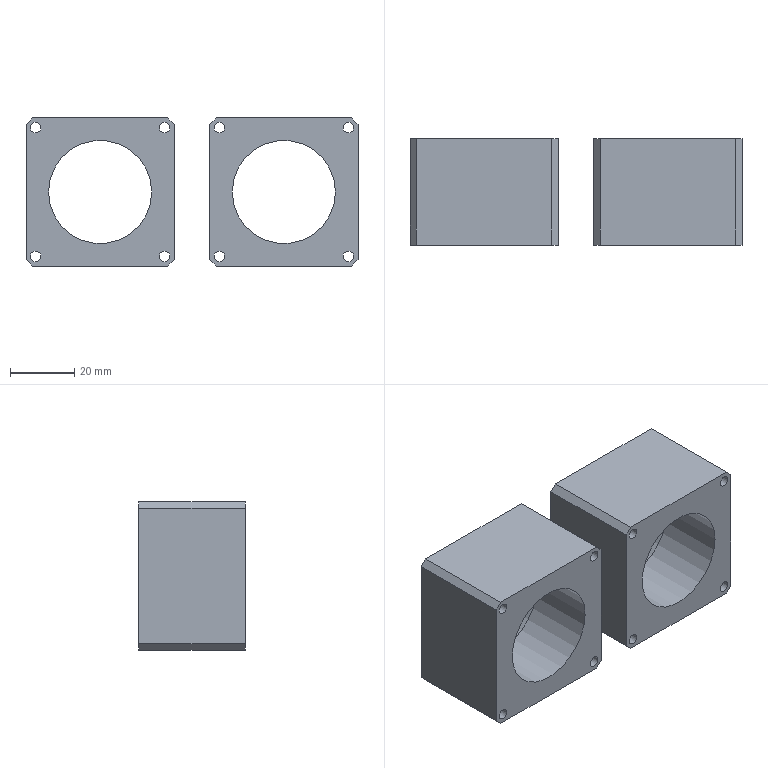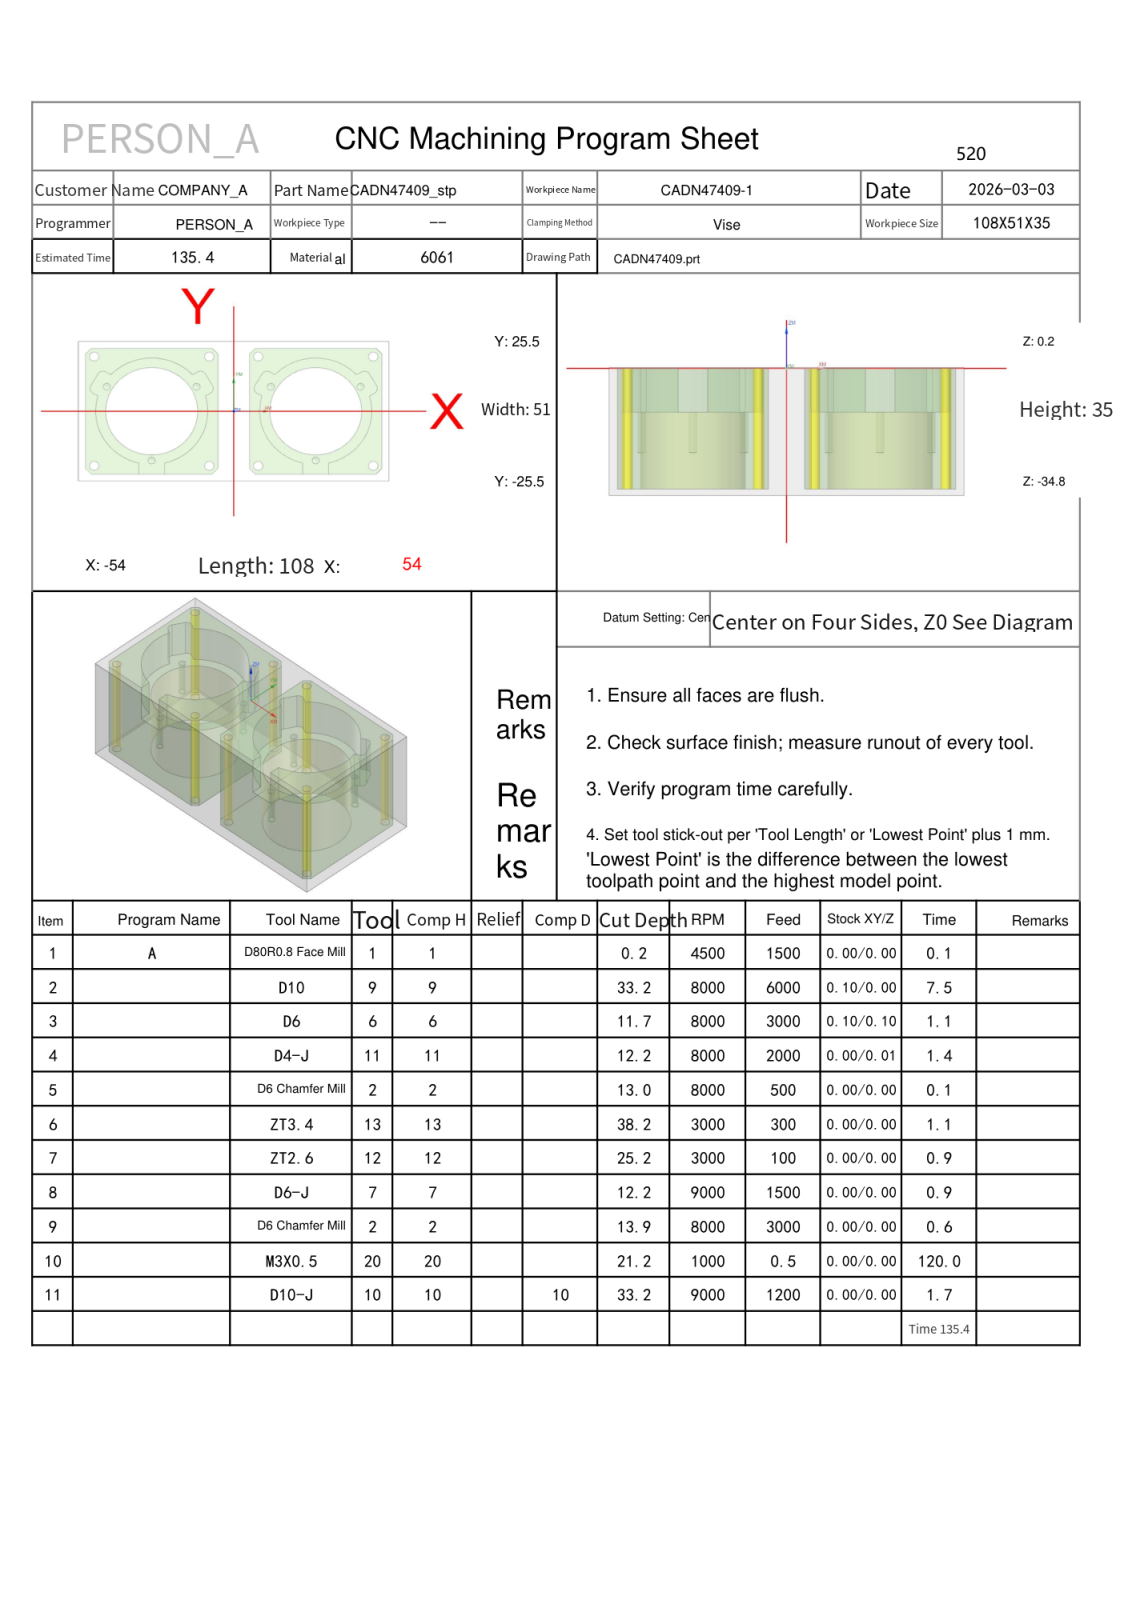NC program | NX | posted by the shop | part box 103 x 33 x 46 mm
Lines 4873 to 5345 of 11287:
N3 T06 M06
(D6  D=6. R=0. H=06 ce=0.10 di=0.10)
G00 G90 G54 X29.9 Y-28.254 M03 S8000
G43 H06 Z50.
M08
Z-.5
G01 Y-23. F3000.
Y-18.974
Y-13.72
G00 Z50.
X27.1
Z-.5
G01 Y-18.974
Y-23.
Y-28.254
G00 Z-1.
G01 Y-23.
Y-18.974
Y-13.72
G00 Z50.
X29.9 Y-28.254
Z-1.
G01 Y-23.
Y-18.974
Y-13.72
G00 Z-1.5
G01 Y-18.974
Y-23.
Y-28.254
G00 Z50.
X27.1 Y-13.72
Z-1.5
G01 Y-18.974
Y-23.
Y-28.254
G00 Z-2.
G01 Y-23.
Y-18.974
Y-13.72
G00 Z50.
X29.9 Y-28.254
Z-2.
G01 Y-23.
Y-18.974
Y-13.72
G00 Z-2.5
G01 Y-18.974
Y-23.
Y-28.254
G00 Z50.
X27.1 Y-13.72
Z-2.5
G01 Y-18.974
Y-23.
Y-28.254
G00 Z-3.
G01 Y-23.
Y-18.974
Y-13.72
G00 Z50.
X29.9 Y-28.254
Z-3.
G01 Y-23.
Y-18.974
Y-13.72
G00 Z-3.5
G01 Y-18.974
Y-23.
Y-28.254
G00 Z50.
X27.1 Y-13.72
Z-3.5
G01 Y-18.974
Y-23.
Y-28.254
G00 Z-4.
G01 Y-23.
Y-18.974
Y-13.72
G00 Z50.
X29.9 Y-28.254
Z-4.
G01 Y-23.
Y-18.974
Y-13.72
G00 Z-4.5
G01 Y-18.974
Y-23.
Y-28.254
G00 Z50.
X27.1 Y-13.72
Z-4.5
G01 Y-18.974
Y-23.
Y-28.254
G00 Z-5.
G01 Y-23.
Y-18.974
Y-13.72
G00 Z50.
X29.9 Y-28.254
Z-5.
G01 Y-23.
Y-18.974
Y-13.72
G00 Z-5.5
G01 Y-18.974
Y-23.
Y-28.254
G00 Z50.
X27.1 Y-13.72
Z-5.5
G01 Y-18.974
Y-23.
Y-28.254
G00 Z-6.
G01 Y-23.
Y-18.974
Y-13.72
G00 Z50.
X29.9 Y-28.254
Z-6.
G01 Y-23.
Y-18.974
Y-13.72
G00 Z-6.5
G01 Y-18.974
Y-23.
Y-28.254
G00 Z50.
X27.1 Y-13.72
Z-6.5
G01 Y-18.974
Y-23.
Y-28.254
G00 Z-7.
G01 Y-23.
Y-18.974
Y-13.72
G00 Z50.
X29.9 Y-28.254
Z-7.
G01 Y-23.
Y-18.974
Y-13.72
G00 Z-7.5
G01 Y-18.974
Y-23.
Y-28.254
G00 Z50.
X27.1 Y-13.72
Z-7.5
G01 Y-18.974
Y-23.
Y-28.254
G00 Z-8.
G01 Y-23.
Y-18.974
Y-13.72
G00 Z50.
X29.9 Y-28.254
Z-8.
G01 Y-23.
Y-18.974
Y-13.72
G00 Z-8.5
G01 Y-18.974
Y-23.
Y-28.254
G00 Z50.
X27.1 Y-13.72
Z-8.5
G01 Y-18.974
Y-23.
Y-28.254
G00 Z-9.
G01 Y-23.
Y-18.974
Y-13.72
G00 Z50.
X29.9 Y-28.254
Z-9.
G01 Y-23.
Y-18.974
Y-13.72
G00 Z-9.5
G01 Y-18.974
Y-23.
Y-28.254
G00 Z50.
X27.1 Y-13.72
Z-9.5
G01 Y-18.974
Y-23.
Y-28.254
G00 Z-10.
G01 Y-23.
Y-18.974
Y-13.72
G00 Z50.
X29.9 Y-28.254
Z-10.
G01 Y-23.
Y-18.974
Y-13.72
G00 Z-10.5
G01 Y-18.974
Y-23.
Y-28.254
G00 Z50.
X27.1 Y-13.72
Z-10.5
G01 Y-18.974
Y-23.
Y-28.254
G00 Z-11.
G01 Y-23.
Y-18.974
Y-13.72
G00 Z50.
X29.9 Y-28.254
Z-11.
G01 Y-23.
Y-18.974
Y-13.72
G00 Z-11.5
G01 Y-18.974
Y-23.
Y-28.254
G00 Z50.
X27.1 Y-13.72
Z-11.5
G01 Y-18.974
Y-23.
Y-28.254
G00 Z50.
X-27.1
Z-.5
G01 Y-23.
Y-18.974
Y-13.72
G00 Z50.
X-29.9
Z-.5
G01 Y-18.974
Y-23.
Y-28.254
G00 Z-1.
G01 Y-23.
Y-18.974
Y-13.72
G00 Z50.
X-27.1 Y-28.254
Z-1.
G01 Y-23.
Y-18.974
Y-13.72
G00 Z-1.5
G01 Y-18.974
Y-23.
Y-28.254
G00 Z50.
X-29.9 Y-13.72
Z-1.5
G01 Y-18.974
Y-23.
Y-28.254
G00 Z-2.
G01 Y-23.
Y-18.974
Y-13.72
G00 Z50.
X-27.1 Y-28.254
Z-2.
G01 Y-23.
Y-18.974
Y-13.72
G00 Z-2.5
G01 Y-18.974
Y-23.
Y-28.254
G00 Z50.
X-29.9 Y-13.72
Z-2.5
G01 Y-18.974
Y-23.
Y-28.254
G00 Z-3.
G01 Y-23.
Y-18.974
Y-13.72
G00 Z50.
X-27.1 Y-28.254
Z-3.
G01 Y-23.
Y-18.974
Y-13.72
G00 Z-3.5
G01 Y-18.974
Y-23.
Y-28.254
G00 Z50.
X-29.9 Y-13.72
Z-3.5
G01 Y-18.974
Y-23.
Y-28.254
G00 Z-4.
G01 Y-23.
Y-18.974
Y-13.72
G00 Z50.
X-27.1 Y-28.254
Z-4.
G01 Y-23.
Y-18.974
Y-13.72
G00 Z-4.5
G01 Y-18.974
Y-23.
Y-28.254
G00 Z50.
X-29.9 Y-13.72
Z-4.5
G01 Y-18.974
Y-23.
Y-28.254
G00 Z-5.
G01 Y-23.
Y-18.974
Y-13.72
G00 Z50.
X-27.1 Y-28.254
Z-5.
G01 Y-23.
Y-18.974
Y-13.72
G00 Z-5.5
G01 Y-18.974
Y-23.
Y-28.254
G00 Z50.
X-29.9 Y-13.72
Z-5.5
G01 Y-18.974
Y-23.
Y-28.254
G00 Z-6.
G01 Y-23.
Y-18.974
Y-13.72
G00 Z50.
X-27.1 Y-28.254
Z-6.
G01 Y-23.
Y-18.974
Y-13.72
G00 Z-6.5
G01 Y-18.974
Y-23.
Y-28.254
G00 Z50.
X-29.9 Y-13.72
Z-6.5
G01 Y-18.974
Y-23.
Y-28.254
G00 Z-7.
G01 Y-23.
Y-18.974
Y-13.72
G00 Z50.
X-27.1 Y-28.254
Z-7.
G01 Y-23.
Y-18.974
Y-13.72
G00 Z-7.5
G01 Y-18.974
Y-23.
Y-28.254
G00 Z50.
X-29.9 Y-13.72
Z-7.5
G01 Y-18.974
Y-23.
Y-28.254
G00 Z-8.
G01 Y-23.
Y-18.974
Y-13.72
G00 Z50.
X-27.1 Y-28.254
Z-8.
G01 Y-23.
Y-18.974
Y-13.72
G00 Z-8.5
G01 Y-18.974
Y-23.
Y-28.254
G00 Z50.
X-29.9 Y-13.72
Z-8.5
G01 Y-18.974
Y-23.
Y-28.254
G00 Z-9.
G01 Y-23.
Y-18.974
Y-13.72
G00 Z50.
X-27.1 Y-28.254
Z-9.
G01 Y-23.
Y-18.974
Y-13.72
G00 Z-9.5
G01 Y-18.974
Y-23.
Y-28.254
G00 Z50.
X-29.9 Y-13.72
Z-9.5
G01 Y-18.974
Y-23.
Y-28.254
G00 Z-10.
G01 Y-23.
Y-18.974
Y-13.72
G00 Z50.
X-27.1 Y-28.254
Z-10.
G01 Y-23.
Y-18.974
Y-13.72
G00 Z-10.5
G01 Y-18.974
Y-23.
Y-28.254
G00 Z50.
X-29.9 Y-13.72
Z-10.5
G01 Y-18.974
Y-23.
Y-28.254
G00 Z-11.
G01 Y-23.
Y-18.974
Y-13.72
G00 Z50.
X-27.1 Y-28.254
Z-11.
G01 Y-23.
Y-18.974
Y-13.72
G00 Z-11.5
G01 Y-18.974
Y-23.
Y-28.254
G00 Z50.
X-29.9 Y-13.72
Z-11.5
G01 Y-18.974
Y-23.
Y-28.254
G00 Z50.
G91 G28 Z0.0
M05
M09
G91 G28 Z0.0
M01